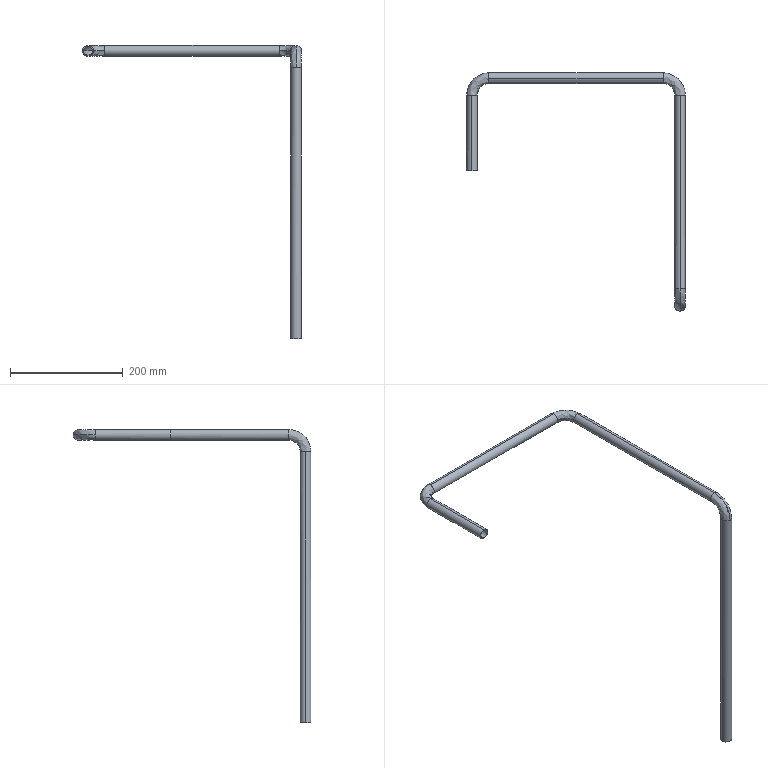Part | STEP file | copper tube 1_default_machined_ | 1 solid | 30 faces | box 388 x 422 x 519.8 mm | volume 116086 mm3 | cylinder 16 | spline 12 | plane 2 | commonest cylinder face diameters 16 x8 19 x8